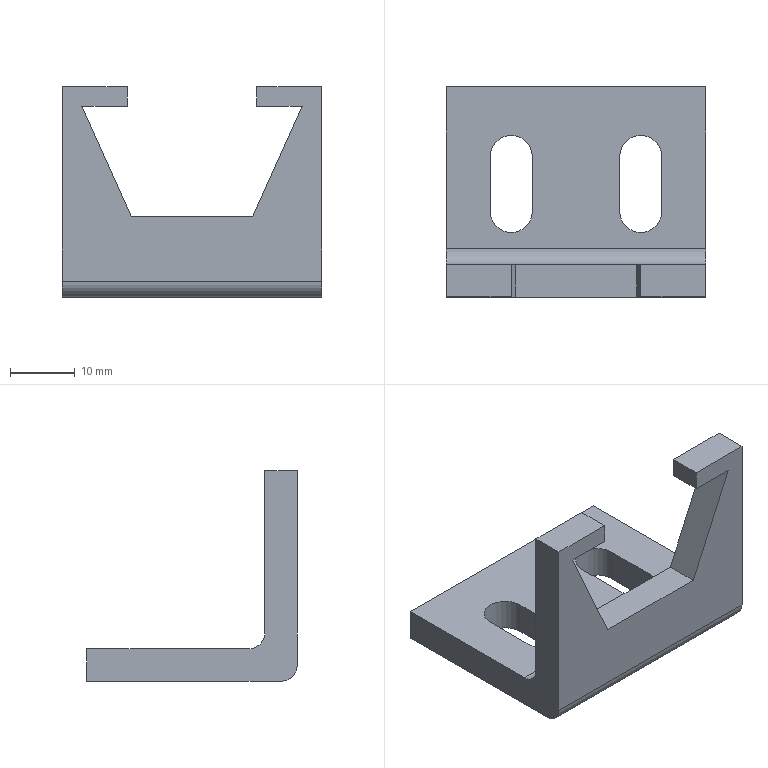Part | SolidWorks | features BaseBody 1 | 1 solid | 26 faces | box 40 x 32.5 x 32.5 mm | volume 8576 mm3 | plane 20 | cylinder 6 | commonest cylinder face diameters 6.5 x4 5 x2
STEP:
#1=CARTESIAN_POINT('',(6.75,5.5,0.));
#2=VERTEX_POINT('',#1);
#3=CARTESIAN_POINT('',(13.25,5.5,0.));
#4=VERTEX_POINT('',#3);
#5=CARTESIAN_POINT('',(10.,5.5,0.));
#6=DIRECTION('',(0.,0.,-1.));
#7=DIRECTION('',(-1.,0.,0.));
#8=AXIS2_PLACEMENT_3D('',#5,#6,#7);
#9=CIRCLE('',#8,3.25);
#10=EDGE_CURVE('',#2,#4,#9,.T.);
#11=ORIENTED_EDGE('',*,*,#10,.F.);
#12=CARTESIAN_POINT('',(6.75,-3.,0.));
#13=VERTEX_POINT('',#12);
#14=CARTESIAN_POINT('',(6.75,-3.,0.));
#15=DIRECTION('',(0.,1.,0.));
#16=VECTOR('',#15,1000.);
#17=LINE('',#14,#16);
#18=EDGE_CURVE('',#13,#2,#17,.T.);
#19=ORIENTED_EDGE('',*,*,#18,.F.);
#20=CARTESIAN_POINT('',(13.25,-3.,0.));
#21=VERTEX_POINT('',#20);
#22=CARTESIAN_POINT('',(10.,-3.,0.));
#23=DIRECTION('',(0.,0.,-1.));
#24=DIRECTION('',(1.,0.,0.));
#25=AXIS2_PLACEMENT_3D('',#22,#23,#24);
#26=CIRCLE('',#25,3.25);
#27=EDGE_CURVE('',#21,#13,#26,.T.);
#28=ORIENTED_EDGE('',*,*,#27,.F.);
#29=CARTESIAN_POINT('',(13.25,5.5,0.));
#30=DIRECTION('',(0.,-1.,0.));
#31=VECTOR('',#30,1000.);
#32=LINE('',#29,#31);
#33=EDGE_CURVE('',#4,#21,#32,.T.);
#34=ORIENTED_EDGE('',*,*,#33,.F.);
#35=EDGE_LOOP('',(#11,#19,#28,#34));
#36=FACE_BOUND('',#35,.T.);
#37=CARTESIAN_POINT('',(-13.25,5.5,0.));
#38=VERTEX_POINT('',#37);
#39=CARTESIAN_POINT('',(-6.75,5.5,0.));
#40=VERTEX_POINT('',#39);
#41=CARTESIAN_POINT('',(-10.,5.5,0.));
#42=DIRECTION('',(0.,0.,-1.));
#43=DIRECTION('',(-1.,0.,0.));
#44=AXIS2_PLACEMENT_3D('',#41,#42,#43);
#45=CIRCLE('',#44,3.25);
#46=EDGE_CURVE('',#38,#40,#45,.T.);
#47=ORIENTED_EDGE('',*,*,#46,.F.);
#48=CARTESIAN_POINT('',(-13.25,-3.,0.));
#49=VERTEX_POINT('',#48);
#50=CARTESIAN_POINT('',(-13.25,-3.,0.));
#51=DIRECTION('',(0.,1.,0.));
#52=VECTOR('',#51,1000.);
#53=LINE('',#50,#52);
#54=EDGE_CURVE('',#49,#38,#53,.T.);
#55=ORIENTED_EDGE('',*,*,#54,.F.);
#56=CARTESIAN_POINT('',(-6.75,-3.,0.));
#57=VERTEX_POINT('',#56);
#58=CARTESIAN_POINT('',(-10.,-3.,0.));
#59=DIRECTION('',(0.,0.,-1.));
#60=DIRECTION('',(1.,0.,0.));
#61=AXIS2_PLACEMENT_3D('',#58,#59,#60);
#62=CIRCLE('',#61,3.25);
#63=EDGE_CURVE('',#57,#49,#62,.T.);
#64=ORIENTED_EDGE('',*,*,#63,.F.);
#65=CARTESIAN_POINT('',(-6.75,5.5,0.));
#66=DIRECTION('',(0.,-1.,0.));
#67=VECTOR('',#66,1000.);
#68=LINE('',#65,#67);
#69=EDGE_CURVE('',#40,#57,#68,.T.);
#70=ORIENTED_EDGE('',*,*,#69,.F.);
#71=EDGE_LOOP('',(#47,#55,#64,#70));
#72=FACE_BOUND('',#71,.T.);
#73=CARTESIAN_POINT('',(-20.,-13.75,0.));
#74=VERTEX_POINT('',#73);
#75=CARTESIAN_POINT('',(20.,-13.75,0.));
#76=VERTEX_POINT('',#75);
#77=CARTESIAN_POINT('',(-20.,-13.75,0.));
#78=DIRECTION('',(1.,0.,0.));
#79=VECTOR('',#78,1000.);
#80=LINE('',#77,#79);
#81=EDGE_CURVE('',#74,#76,#80,.T.);
#82=ORIENTED_EDGE('',*,*,#81,.F.);
#83=CARTESIAN_POINT('',(-20.,16.25,0.));
#84=VERTEX_POINT('',#83);
#85=CARTESIAN_POINT('',(-20.,16.25,0.));
#86=DIRECTION('',(0.,-1.,0.));
#87=VECTOR('',#86,1000.);
#88=LINE('',#85,#87);
#89=EDGE_CURVE('',#84,#74,#88,.T.);
#90=ORIENTED_EDGE('',*,*,#89,.F.);
#91=CARTESIAN_POINT('',(20.,16.25,0.));
#92=VERTEX_POINT('',#91);
#93=CARTESIAN_POINT('',(20.,16.25,0.));
#94=DIRECTION('',(-1.,0.,0.));
#95=VECTOR('',#94,1000.);
#96=LINE('',#93,#95);
#97=EDGE_CURVE('',#92,#84,#96,.T.);
#98=ORIENTED_EDGE('',*,*,#97,.F.);
#99=CARTESIAN_POINT('',(20.,-13.75,0.));
#100=DIRECTION('',(0.,1.,0.));
#101=VECTOR('',#100,1000.);
#102=LINE('',#99,#101);
#103=EDGE_CURVE('',#76,#92,#102,.T.);
#104=ORIENTED_EDGE('',*,*,#103,.F.);
#105=EDGE_LOOP('',(#82,#90,#98,#104));
#106=FACE_OUTER_BOUND('',#105,.T.);
#107=CARTESIAN_POINT('',(0.,0.,0.));
#108=DIRECTION('',(0.,0.,-1.));
#109=DIRECTION('',(0.,-1.,0.));
#110=AXIS2_PLACEMENT_3D('',#107,#108,#109);
#111=PLANE('',#110);
#112=ADVANCED_FACE('',(#36,#72,#106),#111,.T.);
#113=ORIENTED_EDGE('',*,*,#97,.T.);
#114=CARTESIAN_POINT('',(-20.,16.25,5.));
#115=VERTEX_POINT('',#114);
#116=CARTESIAN_POINT('',(-20.,16.25,5.));
#117=DIRECTION('',(0.,0.,-1.));
#118=VECTOR('',#117,1000.);
#119=LINE('',#116,#118);
#120=EDGE_CURVE('',#115,#84,#119,.T.);
#121=ORIENTED_EDGE('',*,*,#120,.F.);
#122=CARTESIAN_POINT('',(20.,16.25,5.));
#123=VERTEX_POINT('',#122);
#124=CARTESIAN_POINT('',(20.,16.25,5.));
#125=DIRECTION('',(-1.,0.,0.));
#126=VECTOR('',#125,1000.);
#127=LINE('',#124,#126);
#128=EDGE_CURVE('',#123,#115,#127,.T.);
#129=ORIENTED_EDGE('',*,*,#128,.F.);
#130=CARTESIAN_POINT('',(20.,16.25,0.));
#131=DIRECTION('',(0.,0.,1.));
#132=VECTOR('',#131,1000.);
#133=LINE('',#130,#132);
#134=EDGE_CURVE('',#92,#123,#133,.T.);
#135=ORIENTED_EDGE('',*,*,#134,.F.);
#136=EDGE_LOOP('',(#113,#121,#129,#135));
#137=FACE_OUTER_BOUND('',#136,.T.);
#138=CARTESIAN_POINT('',(20.,16.25,0.));
#139=DIRECTION('',(0.,1.,0.));
#140=DIRECTION('',(1.,0.,0.));
#141=AXIS2_PLACEMENT_3D('',#138,#139,#140);
#142=PLANE('',#141);
#143=ADVANCED_FACE('',(#137),#142,.T.);
#144=CARTESIAN_POINT('',(-20.,-16.25,2.5));
#145=VERTEX_POINT('',#144);
#146=CARTESIAN_POINT('',(-20.,-13.75,2.5));
#147=DIRECTION('',(1.,0.,0.));
#148=DIRECTION('',(0.,-1.,0.));
#149=AXIS2_PLACEMENT_3D('',#146,#147,#148);
#150=CIRCLE('',#149,2.5);
#151=EDGE_CURVE('',#145,#74,#150,.T.);
#152=ORIENTED_EDGE('',*,*,#151,.F.);
#153=CARTESIAN_POINT('',(-20.,-16.25,32.5));
#154=VERTEX_POINT('',#153);
#155=CARTESIAN_POINT('',(-20.,-16.25,32.5));
#156=DIRECTION('',(0.,0.,-1.));
#157=VECTOR('',#156,1000.);
#158=LINE('',#155,#157);
#159=EDGE_CURVE('',#154,#145,#158,.T.);
#160=ORIENTED_EDGE('',*,*,#159,.F.);
#161=CARTESIAN_POINT('',(-20.,-11.25,32.5));
#162=VERTEX_POINT('',#161);
#163=CARTESIAN_POINT('',(-20.,-11.25,32.5));
#164=DIRECTION('',(0.,-1.,0.));
#165=VECTOR('',#164,1000.);
#166=LINE('',#163,#165);
#167=EDGE_CURVE('',#162,#154,#166,.T.);
#168=ORIENTED_EDGE('',*,*,#167,.F.);
#169=CARTESIAN_POINT('',(-20.,-11.25,7.5));
#170=VERTEX_POINT('',#169);
#171=CARTESIAN_POINT('',(-20.,-11.25,7.5));
#172=DIRECTION('',(0.,0.,1.));
#173=VECTOR('',#172,1000.);
#174=LINE('',#171,#173);
#175=EDGE_CURVE('',#170,#162,#174,.T.);
#176=ORIENTED_EDGE('',*,*,#175,.F.);
#177=CARTESIAN_POINT('',(-20.,-8.75,5.));
#178=VERTEX_POINT('',#177);
#179=CARTESIAN_POINT('',(-20.,-8.75,7.5));
#180=DIRECTION('',(-1.,0.,0.));
#181=DIRECTION('',(0.,0.,-1.));
#182=AXIS2_PLACEMENT_3D('',#179,#180,#181);
#183=CIRCLE('',#182,2.5);
#184=EDGE_CURVE('',#178,#170,#183,.T.);
#185=ORIENTED_EDGE('',*,*,#184,.F.);
#186=CARTESIAN_POINT('',(-20.,16.25,5.));
#187=DIRECTION('',(0.,-1.,0.));
#188=VECTOR('',#187,1000.);
#189=LINE('',#186,#188);
#190=EDGE_CURVE('',#115,#178,#189,.T.);
#191=ORIENTED_EDGE('',*,*,#190,.F.);
#192=ORIENTED_EDGE('',*,*,#120,.T.);
#193=ORIENTED_EDGE('',*,*,#89,.T.);
#194=EDGE_LOOP('',(#152,#160,#168,#176,#185,#191,#192,#193));
#195=FACE_OUTER_BOUND('',#194,.T.);
#196=CARTESIAN_POINT('',(-20.,16.25,0.));
#197=DIRECTION('',(-1.,0.,0.));
#198=DIRECTION('',(0.,0.,1.));
#199=AXIS2_PLACEMENT_3D('',#196,#197,#198);
#200=PLANE('',#199);
#201=ADVANCED_FACE('',(#195),#200,.T.);
#202=ORIENTED_EDGE('',*,*,#10,.T.);
#203=CARTESIAN_POINT('',(13.25,5.5,5.));
#204=VERTEX_POINT('',#203);
#205=CARTESIAN_POINT('',(13.25,5.5,5.));
#206=DIRECTION('',(0.,0.,-1.));
#207=VECTOR('',#206,1000.);
#208=LINE('',#205,#207);
#209=EDGE_CURVE('',#204,#4,#208,.T.);
#210=ORIENTED_EDGE('',*,*,#209,.F.);
#211=CARTESIAN_POINT('',(6.75,5.5,5.));
#212=VERTEX_POINT('',#211);
#213=CARTESIAN_POINT('',(10.,5.5,5.));
#214=DIRECTION('',(0.,0.,-1.));
#215=DIRECTION('',(-1.,0.,0.));
#216=AXIS2_PLACEMENT_3D('',#213,#214,#215);
#217=CIRCLE('',#216,3.25);
#218=EDGE_CURVE('',#212,#204,#217,.T.);
#219=ORIENTED_EDGE('',*,*,#218,.F.);
#220=CARTESIAN_POINT('',(6.75,5.5,0.));
#221=DIRECTION('',(0.,0.,1.));
#222=VECTOR('',#221,1000.);
#223=LINE('',#220,#222);
#224=EDGE_CURVE('',#2,#212,#223,.T.);
#225=ORIENTED_EDGE('',*,*,#224,.F.);
#226=EDGE_LOOP('',(#202,#210,#219,#225));
#227=FACE_OUTER_BOUND('',#226,.T.);
#228=CARTESIAN_POINT('',(10.,5.5,0.));
#229=DIRECTION('',(0.,0.,1.));
#230=DIRECTION('',(1.,0.,0.));
#231=AXIS2_PLACEMENT_3D('',#228,#229,#230);
#232=CYLINDRICAL_SURFACE('',#231,3.25);
#233=ADVANCED_FACE('',(#227),#232,.F.);
#234=ORIENTED_EDGE('',*,*,#33,.T.);
#235=CARTESIAN_POINT('',(13.25,-3.,5.));
#236=VERTEX_POINT('',#235);
#237=CARTESIAN_POINT('',(13.25,-3.,5.));
#238=DIRECTION('',(0.,0.,-1.));
#239=VECTOR('',#238,1000.);
#240=LINE('',#237,#239);
#241=EDGE_CURVE('',#236,#21,#240,.T.);
#242=ORIENTED_EDGE('',*,*,#241,.F.);
#243=CARTESIAN_POINT('',(13.25,5.5,5.));
#244=DIRECTION('',(0.,-1.,0.));
#245=VECTOR('',#244,1000.);
#246=LINE('',#243,#245);
#247=EDGE_CURVE('',#204,#236,#246,.T.);
#248=ORIENTED_EDGE('',*,*,#247,.F.);
#249=ORIENTED_EDGE('',*,*,#209,.T.);
#250=EDGE_LOOP('',(#234,#242,#248,#249));
#251=FACE_OUTER_BOUND('',#250,.T.);
#252=CARTESIAN_POINT('',(13.25,5.5,0.));
#253=DIRECTION('',(-1.,0.,0.));
#254=DIRECTION('',(0.,0.,1.));
#255=AXIS2_PLACEMENT_3D('',#252,#253,#254);
#256=PLANE('',#255);
#257=ADVANCED_FACE('',(#251),#256,.T.);
#258=ORIENTED_EDGE('',*,*,#27,.T.);
#259=CARTESIAN_POINT('',(6.75,-3.,5.));
#260=VERTEX_POINT('',#259);
#261=CARTESIAN_POINT('',(6.75,-3.,5.));
#262=DIRECTION('',(0.,0.,-1.));
#263=VECTOR('',#262,1000.);
#264=LINE('',#261,#263);
#265=EDGE_CURVE('',#260,#13,#264,.T.);
#266=ORIENTED_EDGE('',*,*,#265,.F.);
#267=CARTESIAN_POINT('',(10.,-3.,5.));
#268=DIRECTION('',(0.,0.,-1.));
#269=DIRECTION('',(1.,0.,0.));
#270=AXIS2_PLACEMENT_3D('',#267,#268,#269);
#271=CIRCLE('',#270,3.25);
#272=EDGE_CURVE('',#236,#260,#271,.T.);
#273=ORIENTED_EDGE('',*,*,#272,.F.);
#274=ORIENTED_EDGE('',*,*,#241,.T.);
#275=EDGE_LOOP('',(#258,#266,#273,#274));
#276=FACE_OUTER_BOUND('',#275,.T.);
#277=CARTESIAN_POINT('',(10.,-3.,0.));
#278=DIRECTION('',(0.,0.,1.));
#279=DIRECTION('',(-1.,0.,0.));
#280=AXIS2_PLACEMENT_3D('',#277,#278,#279);
#281=CYLINDRICAL_SURFACE('',#280,3.25);
#282=ADVANCED_FACE('',(#276),#281,.F.);
#283=ORIENTED_EDGE('',*,*,#18,.T.);
#284=ORIENTED_EDGE('',*,*,#224,.T.);
#285=CARTESIAN_POINT('',(6.75,-3.,5.));
#286=DIRECTION('',(0.,1.,0.));
#287=VECTOR('',#286,1000.);
#288=LINE('',#285,#287);
#289=EDGE_CURVE('',#260,#212,#288,.T.);
#290=ORIENTED_EDGE('',*,*,#289,.F.);
#291=ORIENTED_EDGE('',*,*,#265,.T.);
#292=EDGE_LOOP('',(#283,#284,#290,#291));
#293=FACE_OUTER_BOUND('',#292,.T.);
#294=CARTESIAN_POINT('',(6.75,-3.,0.));
#295=DIRECTION('',(1.,0.,0.));
#296=DIRECTION('',(0.,1.,0.));
#297=AXIS2_PLACEMENT_3D('',#294,#295,#296);
#298=PLANE('',#297);
#299=ADVANCED_FACE('',(#293),#298,.T.);
#300=ORIENTED_EDGE('',*,*,#46,.T.);
#301=CARTESIAN_POINT('',(-6.75,5.5,5.));
#302=VERTEX_POINT('',#301);
#303=CARTESIAN_POINT('',(-6.75,5.5,5.));
#304=DIRECTION('',(0.,0.,-1.));
#305=VECTOR('',#304,1000.);
#306=LINE('',#303,#305);
#307=EDGE_CURVE('',#302,#40,#306,.T.);
#308=ORIENTED_EDGE('',*,*,#307,.F.);
#309=CARTESIAN_POINT('',(-13.25,5.5,5.));
#310=VERTEX_POINT('',#309);
#311=CARTESIAN_POINT('',(-10.,5.5,5.));
#312=DIRECTION('',(0.,0.,-1.));
#313=DIRECTION('',(-1.,0.,0.));
#314=AXIS2_PLACEMENT_3D('',#311,#312,#313);
#315=CIRCLE('',#314,3.25);
#316=EDGE_CURVE('',#310,#302,#315,.T.);
#317=ORIENTED_EDGE('',*,*,#316,.F.);
#318=CARTESIAN_POINT('',(-13.25,5.5,0.));
#319=DIRECTION('',(0.,0.,1.));
#320=VECTOR('',#319,1000.);
#321=LINE('',#318,#320);
#322=EDGE_CURVE('',#38,#310,#321,.T.);
#323=ORIENTED_EDGE('',*,*,#322,.F.);
#324=EDGE_LOOP('',(#300,#308,#317,#323));
#325=FACE_OUTER_BOUND('',#324,.T.);
#326=CARTESIAN_POINT('',(-10.,5.5,0.));
#327=DIRECTION('',(0.,0.,1.));
#328=DIRECTION('',(1.,0.,0.));
#329=AXIS2_PLACEMENT_3D('',#326,#327,#328);
#330=CYLINDRICAL_SURFACE('',#329,3.25);
#331=ADVANCED_FACE('',(#325),#330,.F.);
#332=ORIENTED_EDGE('',*,*,#69,.T.);
#333=CARTESIAN_POINT('',(-6.75,-3.,5.));
#334=VERTEX_POINT('',#333);
#335=CARTESIAN_POINT('',(-6.75,-3.,5.));
#336=DIRECTION('',(0.,0.,-1.));
#337=VECTOR('',#336,1000.);
#338=LINE('',#335,#337);
#339=EDGE_CURVE('',#334,#57,#338,.T.);
#340=ORIENTED_EDGE('',*,*,#339,.F.);
#341=CARTESIAN_POINT('',(-6.75,5.5,5.));
#342=DIRECTION('',(0.,-1.,0.));
#343=VECTOR('',#342,1000.);
#344=LINE('',#341,#343);
#345=EDGE_CURVE('',#302,#334,#344,.T.);
#346=ORIENTED_EDGE('',*,*,#345,.F.);
#347=ORIENTED_EDGE('',*,*,#307,.T.);
#348=EDGE_LOOP('',(#332,#340,#346,#347));
#349=FACE_OUTER_BOUND('',#348,.T.);
#350=CARTESIAN_POINT('',(-6.75,5.5,0.));
#351=DIRECTION('',(-1.,0.,0.));
#352=DIRECTION('',(0.,0.,1.));
#353=AXIS2_PLACEMENT_3D('',#350,#351,#352);
#354=PLANE('',#353);
#355=ADVANCED_FACE('',(#349),#354,.T.);
#356=ORIENTED_EDGE('',*,*,#63,.T.);
#357=CARTESIAN_POINT('',(-13.25,-3.,5.));
#358=VERTEX_POINT('',#357);
#359=CARTESIAN_POINT('',(-13.25,-3.,5.));
#360=DIRECTION('',(0.,0.,-1.));
#361=VECTOR('',#360,1000.);
#362=LINE('',#359,#361);
#363=EDGE_CURVE('',#358,#49,#362,.T.);
#364=ORIENTED_EDGE('',*,*,#363,.F.);
#365=CARTESIAN_POINT('',(-10.,-3.,5.));
#366=DIRECTION('',(0.,0.,-1.));
#367=DIRECTION('',(1.,0.,0.));
#368=AXIS2_PLACEMENT_3D('',#365,#366,#367);
#369=CIRCLE('',#368,3.25);
#370=EDGE_CURVE('',#334,#358,#369,.T.);
#371=ORIENTED_EDGE('',*,*,#370,.F.);
#372=ORIENTED_EDGE('',*,*,#339,.T.);
#373=EDGE_LOOP('',(#356,#364,#371,#372));
#374=FACE_OUTER_BOUND('',#373,.T.);
#375=CARTESIAN_POINT('',(-10.,-3.,0.));
#376=DIRECTION('',(0.,0.,1.));
#377=DIRECTION('',(-1.,0.,0.));
#378=AXIS2_PLACEMENT_3D('',#375,#376,#377);
#379=CYLINDRICAL_SURFACE('',#378,3.25);
#380=ADVANCED_FACE('',(#374),#379,.F.);
#381=ORIENTED_EDGE('',*,*,#54,.T.);
#382=ORIENTED_EDGE('',*,*,#322,.T.);
#383=CARTESIAN_POINT('',(-13.25,-3.,5.));
#384=DIRECTION('',(0.,1.,0.));
#385=VECTOR('',#384,1000.);
#386=LINE('',#383,#385);
#387=EDGE_CURVE('',#358,#310,#386,.T.);
#388=ORIENTED_EDGE('',*,*,#387,.F.);
#389=ORIENTED_EDGE('',*,*,#363,.T.);
#390=EDGE_LOOP('',(#381,#382,#388,#389));
#391=FACE_OUTER_BOUND('',#390,.T.);
#392=CARTESIAN_POINT('',(-13.25,-3.,0.));
#393=DIRECTION('',(1.,0.,0.));
#394=DIRECTION('',(0.,1.,0.));
#395=AXIS2_PLACEMENT_3D('',#392,#393,#394);
#396=PLANE('',#395);
#397=ADVANCED_FACE('',(#391),#396,.T.);
#398=ORIENTED_EDGE('',*,*,#316,.T.);
#399=ORIENTED_EDGE('',*,*,#345,.T.);
#400=ORIENTED_EDGE('',*,*,#370,.T.);
#401=ORIENTED_EDGE('',*,*,#387,.T.);
#402=EDGE_LOOP('',(#398,#399,#400,#401));
#403=FACE_BOUND('',#402,.T.);
#404=ORIENTED_EDGE('',*,*,#218,.T.);
#405=ORIENTED_EDGE('',*,*,#247,.T.);
#406=ORIENTED_EDGE('',*,*,#272,.T.);
#407=ORIENTED_EDGE('',*,*,#289,.T.);
#408=EDGE_LOOP('',(#404,#405,#406,#407));
#409=FACE_BOUND('',#408,.T.);
#410=CARTESIAN_POINT('',(20.,-8.75,5.));
#411=VERTEX_POINT('',#410);
#412=CARTESIAN_POINT('',(20.,-8.75,5.));
#413=DIRECTION('',(-1.,0.,0.));
#414=VECTOR('',#413,1000.);
#415=LINE('',#412,#414);
#416=EDGE_CURVE('',#411,#178,#415,.T.);
#417=ORIENTED_EDGE('',*,*,#416,.F.);
#418=CARTESIAN_POINT('',(20.,16.25,5.));
#419=DIRECTION('',(0.,-1.,0.));
#420=VECTOR('',#419,1000.);
#421=LINE('',#418,#420);
#422=EDGE_CURVE('',#123,#411,#421,.T.);
#423=ORIENTED_EDGE('',*,*,#422,.F.);
#424=ORIENTED_EDGE('',*,*,#128,.T.);
#425=ORIENTED_EDGE('',*,*,#190,.T.);
#426=EDGE_LOOP('',(#417,#423,#424,#425));
#427=FACE_OUTER_BOUND('',#426,.T.);
#428=CARTESIAN_POINT('',(0.,0.,5.));
#429=DIRECTION('',(0.,0.,1.));
#430=DIRECTION('',(1.,0.,0.));
#431=AXIS2_PLACEMENT_3D('',#428,#429,#430);
#432=PLANE('',#431);
#433=ADVANCED_FACE('',(#403,#409,#427),#432,.T.);
#434=CARTESIAN_POINT('',(-10.,-16.25,32.5));
#435=VERTEX_POINT('',#434);
#436=CARTESIAN_POINT('',(-10.,-16.25,32.5));
#437=DIRECTION('',(-1.,0.,0.));
#438=VECTOR('',#437,1000.);
#439=LINE('',#436,#438);
#440=EDGE_CURVE('',#435,#154,#439,.T.);
#441=ORIENTED_EDGE('',*,*,#440,.F.);
#442=CARTESIAN_POINT('',(-10.,-11.25,32.5));
#443=VERTEX_POINT('',#442);
#444=CARTESIAN_POINT('',(-10.,-11.25,32.5));
#445=DIRECTION('',(0.,-1.,0.));
#446=VECTOR('',#445,1000.);
#447=LINE('',#444,#446);
#448=EDGE_CURVE('',#443,#435,#447,.T.);
#449=ORIENTED_EDGE('',*,*,#448,.F.);
#450=CARTESIAN_POINT('',(-20.,-11.25,32.5));
#451=DIRECTION('',(1.,0.,0.));
#452=VECTOR('',#451,1000.);
#453=LINE('',#450,#452);
#454=EDGE_CURVE('',#162,#443,#453,.T.);
#455=ORIENTED_EDGE('',*,*,#454,.F.);
#456=ORIENTED_EDGE('',*,*,#167,.T.);
#457=EDGE_LOOP('',(#441,#449,#455,#456));
#458=FACE_OUTER_BOUND('',#457,.T.);
#459=CARTESIAN_POINT('',(-20.,-16.25,32.5));
#460=DIRECTION('',(0.,0.,1.));
#461=DIRECTION('',(1.,0.,0.));
#462=AXIS2_PLACEMENT_3D('',#459,#460,#461);
#463=PLANE('',#462);
#464=ADVANCED_FACE('',(#458),#463,.T.);
#465=CARTESIAN_POINT('',(-10.,-16.25,29.5));
#466=VERTEX_POINT('',#465);
#467=CARTESIAN_POINT('',(-10.,-16.25,29.5));
#468=DIRECTION('',(0.,0.,1.));
#469=VECTOR('',#468,1000.);
#470=LINE('',#467,#469);
#471=EDGE_CURVE('',#466,#435,#470,.T.);
#472=ORIENTED_EDGE('',*,*,#471,.F.);
#473=CARTESIAN_POINT('',(-10.,-11.25,29.5));
#474=VERTEX_POINT('',#473);
#475=CARTESIAN_POINT('',(-10.,-11.25,29.5));
#476=DIRECTION('',(0.,-1.,0.));
#477=VECTOR('',#476,1000.);
#478=LINE('',#475,#477);
#479=EDGE_CURVE('',#474,#466,#478,.T.);
#480=ORIENTED_EDGE('',*,*,#479,.F.);
#481=CARTESIAN_POINT('',(-10.,-11.25,32.5));
#482=DIRECTION('',(0.,0.,-1.));
#483=VECTOR('',#482,1000.);
#484=LINE('',#481,#483);
#485=EDGE_CURVE('',#443,#474,#484,.T.);
#486=ORIENTED_EDGE('',*,*,#485,.F.);
#487=ORIENTED_EDGE('',*,*,#448,.T.);
#488=EDGE_LOOP('',(#472,#480,#486,#487));
#489=FACE_OUTER_BOUND('',#488,.T.);
#490=CARTESIAN_POINT('',(-10.,-16.25,32.5));
#491=DIRECTION('',(1.,0.,0.));
#492=DIRECTION('',(0.,1.,0.));
#493=AXIS2_PLACEMENT_3D('',#490,#491,#492);
#494=PLANE('',#493);
#495=ADVANCED_FACE('',(#489),#494,.T.);
#496=CARTESIAN_POINT('',(-17.,-16.25,29.5));
#497=VERTEX_POINT('',#496);
#498=CARTESIAN_POINT('',(-17.,-16.25,29.5));
#499=DIRECTION('',(1.,0.,0.));
#500=VECTOR('',#499,1000.);
#501=LINE('',#498,#500);
#502=EDGE_CURVE('',#497,#466,#501,.T.);
#503=ORIENTED_EDGE('',*,*,#502,.F.);
#504=CARTESIAN_POINT('',(-17.,-11.25,29.5));
#505=VERTEX_POINT('',#504);
#506=CARTESIAN_POINT('',(-17.,-11.25,29.5));
#507=DIRECTION('',(0.,-1.,0.));
#508=VECTOR('',#507,1000.);
#509=LINE('',#506,#508);
#510=EDGE_CURVE('',#505,#497,#509,.T.);
#511=ORIENTED_EDGE('',*,*,#510,.F.);
#512=CARTESIAN_POINT('',(-10.,-11.25,29.5));
#513=DIRECTION('',(-1.,0.,0.));
#514=VECTOR('',#513,1000.);
#515=LINE('',#512,#514);
#516=EDGE_CURVE('',#474,#505,#515,.T.);
#517=ORIENTED_EDGE('',*,*,#516,.F.);
#518=ORIENTED_EDGE('',*,*,#479,.T.);
#519=EDGE_LOOP('',(#503,#511,#517,#518));
#520=FACE_OUTER_BOUND('',#519,.T.);
#521=CARTESIAN_POINT('',(-10.,-16.25,29.5));
#522=DIRECTION('',(0.,0.,-1.));
#523=DIRECTION('',(0.,-1.,0.));
#524=AXIS2_PLACEMENT_3D('',#521,#522,#523);
#525=PLANE('',#524);
#526=ADVANCED_FACE('',(#520),#525,.T.);
#527=CARTESIAN_POINT('',(-9.35,-16.25,12.5));
#528=VERTEX_POINT('',#527);
#529=CARTESIAN_POINT('',(-9.35,-16.25,12.5));
#530=DIRECTION('',(-0.4104,0.,0.9119));
#531=VECTOR('',#530,1000.);
#532=LINE('',#529,#531);
#533=EDGE_CURVE('',#528,#497,#532,.T.);
#534=ORIENTED_EDGE('',*,*,#533,.F.);
#535=CARTESIAN_POINT('',(-9.35,-11.25,12.5));
#536=VERTEX_POINT('',#535);
#537=CARTESIAN_POINT('',(-9.35,-11.25,12.5));
#538=DIRECTION('',(0.,-1.,0.));
#539=VECTOR('',#538,1000.);
#540=LINE('',#537,#539);
#541=EDGE_CURVE('',#536,#528,#540,.T.);
#542=ORIENTED_EDGE('',*,*,#541,.F.);
#543=CARTESIAN_POINT('',(-17.,-11.25,29.5));
#544=DIRECTION('',(0.4104,0.,-0.9119));
#545=VECTOR('',#544,1000.);
#546=LINE('',#543,#545);
#547=EDGE_CURVE('',#505,#536,#546,.T.);
#548=ORIENTED_EDGE('',*,*,#547,.F.);
#549=ORIENTED_EDGE('',*,*,#510,.T.);
#550=EDGE_LOOP('',(#534,#542,#548,#549));
#551=FACE_OUTER_BOUND('',#550,.T.);
#552=CARTESIAN_POINT('',(-17.,-16.25,29.5));
#553=DIRECTION('',(0.9119,0.,0.4104));
#554=DIRECTION('',(0.,-1.,0.));
#555=AXIS2_PLACEMENT_3D('',#552,#553,#554);
#556=PLANE('',#555);
#557=ADVANCED_FACE('',(#551),#556,.T.);
#558=CARTESIAN_POINT('',(9.35,-16.25,12.5));
#559=VERTEX_POINT('',#558);
#560=CARTESIAN_POINT('',(9.35,-16.25,12.5));
#561=DIRECTION('',(-1.,0.,0.));
#562=VECTOR('',#561,1000.);
#563=LINE('',#560,#562);
#564=EDGE_CURVE('',#559,#528,#563,.T.);
#565=ORIENTED_EDGE('',*,*,#564,.F.);
#566=CARTESIAN_POINT('',(9.35,-11.25,12.5));
#567=VERTEX_POINT('',#566);
#568=CARTESIAN_POINT('',(9.35,-11.25,12.5));
#569=DIRECTION('',(0.,-1.,0.));
#570=VECTOR('',#569,1000.);
#571=LINE('',#568,#570);
#572=EDGE_CURVE('',#567,#559,#571,.T.);
#573=ORIENTED_EDGE('',*,*,#572,.F.);
#574=CARTESIAN_POINT('',(-9.35,-11.25,12.5));
#575=DIRECTION('',(1.,0.,0.));
#576=VECTOR('',#575,1000.);
#577=LINE('',#574,#576);
#578=EDGE_CURVE('',#536,#567,#577,.T.);
#579=ORIENTED_EDGE('',*,*,#578,.F.);
#580=ORIENTED_EDGE('',*,*,#541,.T.);
#581=EDGE_LOOP('',(#565,#573,#579,#580));
#582=FACE_OUTER_BOUND('',#581,.T.);
#583=CARTESIAN_POINT('',(-9.35,-16.25,12.5));
#584=DIRECTION('',(0.,0.,1.));
#585=DIRECTION('',(1.,0.,0.));
#586=AXIS2_PLACEMENT_3D('',#583,#584,#585);
#587=PLANE('',#586);
#588=ADVANCED_FACE('',(#582),#587,.T.);
#589=CARTESIAN_POINT('',(17.,-16.25,29.5));
#590=VERTEX_POINT('',#589);
#591=CARTESIAN_POINT('',(17.,-16.25,29.5));
#592=DIRECTION('',(-0.4104,0.,-0.9119));
#593=VECTOR('',#592,1000.);
#594=LINE('',#591,#593);
#595=EDGE_CURVE('',#590,#559,#594,.T.);
#596=ORIENTED_EDGE('',*,*,#595,.F.);
#597=CARTESIAN_POINT('',(17.,-11.25,29.5));
#598=VERTEX_POINT('',#597);
#599=CARTESIAN_POINT('',(17.,-11.25,29.5));
#600=DIRECTION('',(0.,-1.,0.));
#601=VECTOR('',#600,1000.);
#602=LINE('',#599,#601);
#603=EDGE_CURVE('',#598,#590,#602,.T.);
#604=ORIENTED_EDGE('',*,*,#603,.F.);
#605=CARTESIAN_POINT('',(9.35,-11.25,12.5));
#606=DIRECTION('',(0.4104,0.,0.9119));
#607=VECTOR('',#606,1000.);
#608=LINE('',#605,#607);
#609=EDGE_CURVE('',#567,#598,#608,.T.);
#610=ORIENTED_EDGE('',*,*,#609,.F.);
#611=ORIENTED_EDGE('',*,*,#572,.T.);
#612=EDGE_LOOP('',(#596,#604,#610,#611));
#613=FACE_OUTER_BOUND('',#612,.T.);
#614=CARTESIAN_POINT('',(9.35,-16.25,12.5));
#615=DIRECTION('',(-0.9119,0.,0.4104));
#616=DIRECTION('',(0.,1.,0.));
#617=AXIS2_PLACEMENT_3D('',#614,#615,#616);
#618=PLANE('',#617);
#619=ADVANCED_FACE('',(#613),#618,.T.);
#620=CARTESIAN_POINT('',(10.,-16.25,29.5));
#621=VERTEX_POINT('',#620);
#622=CARTESIAN_POINT('',(10.,-16.25,29.5));
#623=DIRECTION('',(1.,0.,0.));
#624=VECTOR('',#623,1000.);
#625=LINE('',#622,#624);
#626=EDGE_CURVE('',#621,#590,#625,.T.);
#627=ORIENTED_EDGE('',*,*,#626,.F.);
#628=CARTESIAN_POINT('',(10.,-11.25,29.5));
#629=VERTEX_POINT('',#628);
#630=CARTESIAN_POINT('',(10.,-11.25,29.5));
#631=DIRECTION('',(0.,-1.,0.));
#632=VECTOR('',#631,1000.);
#633=LINE('',#630,#632);
#634=EDGE_CURVE('',#629,#621,#633,.T.);
#635=ORIENTED_EDGE('',*,*,#634,.F.);
#636=CARTESIAN_POINT('',(17.,-11.25,29.5));
#637=DIRECTION('',(-1.,0.,0.));
#638=VECTOR('',#637,1000.);
#639=LINE('',#636,#638);
#640=EDGE_CURVE('',#598,#629,#639,.T.);
#641=ORIENTED_EDGE('',*,*,#640,.F.);
#642=ORIENTED_EDGE('',*,*,#603,.T.);
#643=EDGE_LOOP('',(#627,#635,#641,#642));
#644=FACE_OUTER_BOUND('',#643,.T.);
#645=CARTESIAN_POINT('',(17.,-16.25,29.5));
#646=DIRECTION('',(0.,0.,-1.));
#647=DIRECTION('',(-1.,0.,0.));
#648=AXIS2_PLACEMENT_3D('',#645,#646,#647);
#649=PLANE('',#648);
#650=ADVANCED_FACE('',(#644),#649,.T.);
#651=CARTESIAN_POINT('',(10.,-16.25,32.5));
#652=VERTEX_POINT('',#651);
#653=CARTESIAN_POINT('',(10.,-16.25,32.5));
#654=DIRECTION('',(0.,0.,-1.));
#655=VECTOR('',#654,1000.);
#656=LINE('',#653,#655);
#657=EDGE_CURVE('',#652,#621,#656,.T.);
#658=ORIENTED_EDGE('',*,*,#657,.F.);
#659=CARTESIAN_POINT('',(10.,-11.25,32.5));
#660=VERTEX_POINT('',#659);
#661=CARTESIAN_POINT('',(10.,-11.25,32.5));
#662=DIRECTION('',(0.,-1.,0.));
#663=VECTOR('',#662,1000.);
#664=LINE('',#661,#663);
#665=EDGE_CURVE('',#660,#652,#664,.T.);
#666=ORIENTED_EDGE('',*,*,#665,.F.);
#667=CARTESIAN_POINT('',(10.,-11.25,29.5));
#668=DIRECTION('',(0.,0.,1.));
#669=VECTOR('',#668,1000.);
#670=LINE('',#667,#669);
#671=EDGE_CURVE('',#629,#660,#670,.T.);
#672=ORIENTED_EDGE('',*,*,#671,.F.);
#673=ORIENTED_EDGE('',*,*,#634,.T.);
#674=EDGE_LOOP('',(#658,#666,#672,#673));
#675=FACE_OUTER_BOUND('',#674,.T.);
#676=CARTESIAN_POINT('',(10.,-16.25,29.5));
#677=DIRECTION('',(-1.,0.,0.));
#678=DIRECTION('',(0.,0.,1.));
#679=AXIS2_PLACEMENT_3D('',#676,#677,#678);
#680=PLANE('',#679);
#681=ADVANCED_FACE('',(#675),#680,.T.);
#682=CARTESIAN_POINT('',(20.,-16.25,32.5));
#683=VERTEX_POINT('',#682);
#684=CARTESIAN_POINT('',(20.,-16.25,32.5));
#685=DIRECTION('',(-1.,0.,0.));
#686=VECTOR('',#685,1000.);
#687=LINE('',#684,#686);
#688=EDGE_CURVE('',#683,#652,#687,.T.);
#689=ORIENTED_EDGE('',*,*,#688,.F.);
#690=CARTESIAN_POINT('',(20.,-11.25,32.5));
#691=VERTEX_POINT('',#690);
#692=CARTESIAN_POINT('',(20.,-11.25,32.5));
#693=DIRECTION('',(0.,-1.,0.));
#694=VECTOR('',#693,1000.);
#695=LINE('',#692,#694);
#696=EDGE_CURVE('',#691,#683,#695,.T.);
#697=ORIENTED_EDGE('',*,*,#696,.F.);
#698=CARTESIAN_POINT('',(10.,-11.25,32.5));
#699=DIRECTION('',(1.,0.,0.));
#700=VECTOR('',#699,1000.);
#701=LINE('',#698,#700);
#702=EDGE_CURVE('',#660,#691,#701,.T.);
#703=ORIENTED_EDGE('',*,*,#702,.F.);
#704=ORIENTED_EDGE('',*,*,#665,.T.);
#705=EDGE_LOOP('',(#689,#697,#703,#704));
#706=FACE_OUTER_BOUND('',#705,.T.);
#707=CARTESIAN_POINT('',(10.,-16.25,32.5));
#708=DIRECTION('',(0.,0.,1.));
#709=DIRECTION('',(1.,0.,0.));
#710=AXIS2_PLACEMENT_3D('',#707,#708,#709);
#711=PLANE('',#710);
#712=ADVANCED_FACE('',(#706),#711,.T.);
#713=CARTESIAN_POINT('',(20.,-16.25,2.5));
#714=VERTEX_POINT('',#713);
#715=CARTESIAN_POINT('',(20.,-13.75,2.5));
#716=DIRECTION('',(-1.,0.,0.));
#717=DIRECTION('',(0.,0.,-1.));
#718=AXIS2_PLACEMENT_3D('',#715,#716,#717);
#719=CIRCLE('',#718,2.5);
#720=EDGE_CURVE('',#76,#714,#719,.T.);
#721=ORIENTED_EDGE('',*,*,#720,.F.);
#722=ORIENTED_EDGE('',*,*,#103,.T.);
#723=ORIENTED_EDGE('',*,*,#134,.T.);
#724=ORIENTED_EDGE('',*,*,#422,.T.);
#725=CARTESIAN_POINT('',(20.,-11.25,7.5));
#726=VERTEX_POINT('',#725);
#727=CARTESIAN_POINT('',(20.,-8.75,7.5));
#728=DIRECTION('',(1.,0.,0.));
#729=DIRECTION('',(0.,-1.,0.));
#730=AXIS2_PLACEMENT_3D('',#727,#728,#729);
#731=CIRCLE('',#730,2.5);
#732=EDGE_CURVE('',#726,#411,#731,.T.);
#733=ORIENTED_EDGE('',*,*,#732,.F.);
#734=CARTESIAN_POINT('',(20.,-11.25,32.5));
#735=DIRECTION('',(0.,0.,-1.));
#736=VECTOR('',#735,1000.);
#737=LINE('',#734,#736);
#738=EDGE_CURVE('',#691,#726,#737,.T.);
#739=ORIENTED_EDGE('',*,*,#738,.F.);
#740=ORIENTED_EDGE('',*,*,#696,.T.);
#741=CARTESIAN_POINT('',(20.,-16.25,2.5));
#742=DIRECTION('',(0.,0.,1.));
#743=VECTOR('',#742,1000.);
#744=LINE('',#741,#743);
#745=EDGE_CURVE('',#714,#683,#744,.T.);
#746=ORIENTED_EDGE('',*,*,#745,.F.);
#747=EDGE_LOOP('',(#721,#722,#723,#724,#733,#739,#740,#746));
#748=FACE_OUTER_BOUND('',#747,.T.);
#749=CARTESIAN_POINT('',(20.,-16.25,0.));
#750=DIRECTION('',(1.,0.,0.));
#751=DIRECTION('',(0.,1.,0.));
#752=AXIS2_PLACEMENT_3D('',#749,#750,#751);
#753=PLANE('',#752);
#754=ADVANCED_FACE('',(#748),#753,.T.);
#755=CARTESIAN_POINT('',(20.,-16.25,2.5));
#756=DIRECTION('',(-1.,0.,0.));
#757=VECTOR('',#756,1000.);
#758=LINE('',#755,#757);
#759=EDGE_CURVE('',#714,#145,#758,.T.);
#760=ORIENTED_EDGE('',*,*,#759,.F.);
#761=ORIENTED_EDGE('',*,*,#745,.T.);
#762=ORIENTED_EDGE('',*,*,#688,.T.);
#763=ORIENTED_EDGE('',*,*,#657,.T.);
#764=ORIENTED_EDGE('',*,*,#626,.T.);
#765=ORIENTED_EDGE('',*,*,#595,.T.);
#766=ORIENTED_EDGE('',*,*,#564,.T.);
#767=ORIENTED_EDGE('',*,*,#533,.T.);
#768=ORIENTED_EDGE('',*,*,#502,.T.);
#769=ORIENTED_EDGE('',*,*,#471,.T.);
#770=ORIENTED_EDGE('',*,*,#440,.T.);
#771=ORIENTED_EDGE('',*,*,#159,.T.);
#772=EDGE_LOOP('',(#760,#761,#762,#763,#764,#765,#766,#767,#768,#769,#770,#771));
#773=FACE_OUTER_BOUND('',#772,.T.);
#774=CARTESIAN_POINT('',(-20.,-16.25,0.));
#775=DIRECTION('',(0.,-1.,0.));
#776=DIRECTION('',(0.,0.,-1.));
#777=AXIS2_PLACEMENT_3D('',#774,#775,#776);
#778=PLANE('',#777);
#779=ADVANCED_FACE('',(#773),#778,.T.);
#780=ORIENTED_EDGE('',*,*,#151,.T.);
#781=ORIENTED_EDGE('',*,*,#81,.T.);
#782=ORIENTED_EDGE('',*,*,#720,.T.);
#783=ORIENTED_EDGE('',*,*,#759,.T.);
#784=EDGE_LOOP('',(#780,#781,#782,#783));
#785=FACE_OUTER_BOUND('',#784,.T.);
#786=CARTESIAN_POINT('',(20.,-13.75,2.5));
#787=DIRECTION('',(-1.,0.,0.));
#788=DIRECTION('',(0.,-1.,0.));
#789=AXIS2_PLACEMENT_3D('',#786,#787,#788);
#790=CYLINDRICAL_SURFACE('',#789,2.5);
#791=ADVANCED_FACE('',(#785),#790,.T.);
#792=CARTESIAN_POINT('',(-20.,-11.25,7.5));
#793=DIRECTION('',(1.,0.,0.));
#794=VECTOR('',#793,1000.);
#795=LINE('',#792,#794);
#796=EDGE_CURVE('',#170,#726,#795,.T.);
#797=ORIENTED_EDGE('',*,*,#796,.F.);
#798=ORIENTED_EDGE('',*,*,#175,.T.);
#799=ORIENTED_EDGE('',*,*,#454,.T.);
#800=ORIENTED_EDGE('',*,*,#485,.T.);
#801=ORIENTED_EDGE('',*,*,#516,.T.);
#802=ORIENTED_EDGE('',*,*,#547,.T.);
#803=ORIENTED_EDGE('',*,*,#578,.T.);
#804=ORIENTED_EDGE('',*,*,#609,.T.);
#805=ORIENTED_EDGE('',*,*,#640,.T.);
#806=ORIENTED_EDGE('',*,*,#671,.T.);
#807=ORIENTED_EDGE('',*,*,#702,.T.);
#808=ORIENTED_EDGE('',*,*,#738,.T.);
#809=EDGE_LOOP('',(#797,#798,#799,#800,#801,#802,#803,#804,#805,#806,#807,#808));
#810=FACE_OUTER_BOUND('',#809,.T.);
#811=CARTESIAN_POINT('',(0.,-11.25,18.75));
#812=DIRECTION('',(0.,1.,0.));
#813=DIRECTION('',(1.,0.,0.));
#814=AXIS2_PLACEMENT_3D('',#811,#812,#813);
#815=PLANE('',#814);
#816=ADVANCED_FACE('',(#810),#815,.T.);
#817=ORIENTED_EDGE('',*,*,#184,.T.);
#818=ORIENTED_EDGE('',*,*,#796,.T.);
#819=ORIENTED_EDGE('',*,*,#732,.T.);
#820=ORIENTED_EDGE('',*,*,#416,.T.);
#821=EDGE_LOOP('',(#817,#818,#819,#820));
#822=FACE_OUTER_BOUND('',#821,.T.);
#823=CARTESIAN_POINT('',(-20.,-8.75,7.5));
#824=DIRECTION('',(1.,0.,0.));
#825=DIRECTION('',(0.,-1.,0.000000365));
#826=AXIS2_PLACEMENT_3D('',#823,#824,#825);
#827=CYLINDRICAL_SURFACE('',#826,2.5);
#828=ADVANCED_FACE('',(#822),#827,.F.);
#829=CLOSED_SHELL('',(#112,#143,#201,#233,#257,#282,#299,#331,#355,#380,#397,#433,#464,#495,#526,#557,#588,#619,#650,#681,#712,#754,#779,#791,#816,#828));
#830=MANIFOLD_SOLID_BREP('',#829);
#831=CARTESIAN_POINT('',(0.,0.,0.));
#832=DIRECTION('',(0.,0.,1.));
#833=DIRECTION('',(1.,0.,0.));
#834=AXIS2_PLACEMENT_3D('',#831,#832,#833);
#835=(LENGTH_UNIT()NAMED_UNIT(*)SI_UNIT(.MILLI.,.METRE.));
#836=UNCERTAINTY_MEASURE_WITH_UNIT(LENGTH_MEASURE(0.00001),#835,'','');
#837=(NAMED_UNIT(*)PLANE_ANGLE_UNIT()SI_UNIT($,.RADIAN.));
#838=(NAMED_UNIT(*)SI_UNIT($,.STERADIAN.)SOLID_ANGLE_UNIT());
#839=(GEOMETRIC_REPRESENTATION_CONTEXT(3)GLOBAL_UNCERTAINTY_ASSIGNED_CONTEXT((#836))GLOBAL_UNIT_ASSIGNED_CONTEXT((#835,#837,#838))REPRESENTATION_CONTEXT('',''));
#840=ADVANCED_BREP_SHAPE_REPRESENTATION('',(#830,#834),#839);